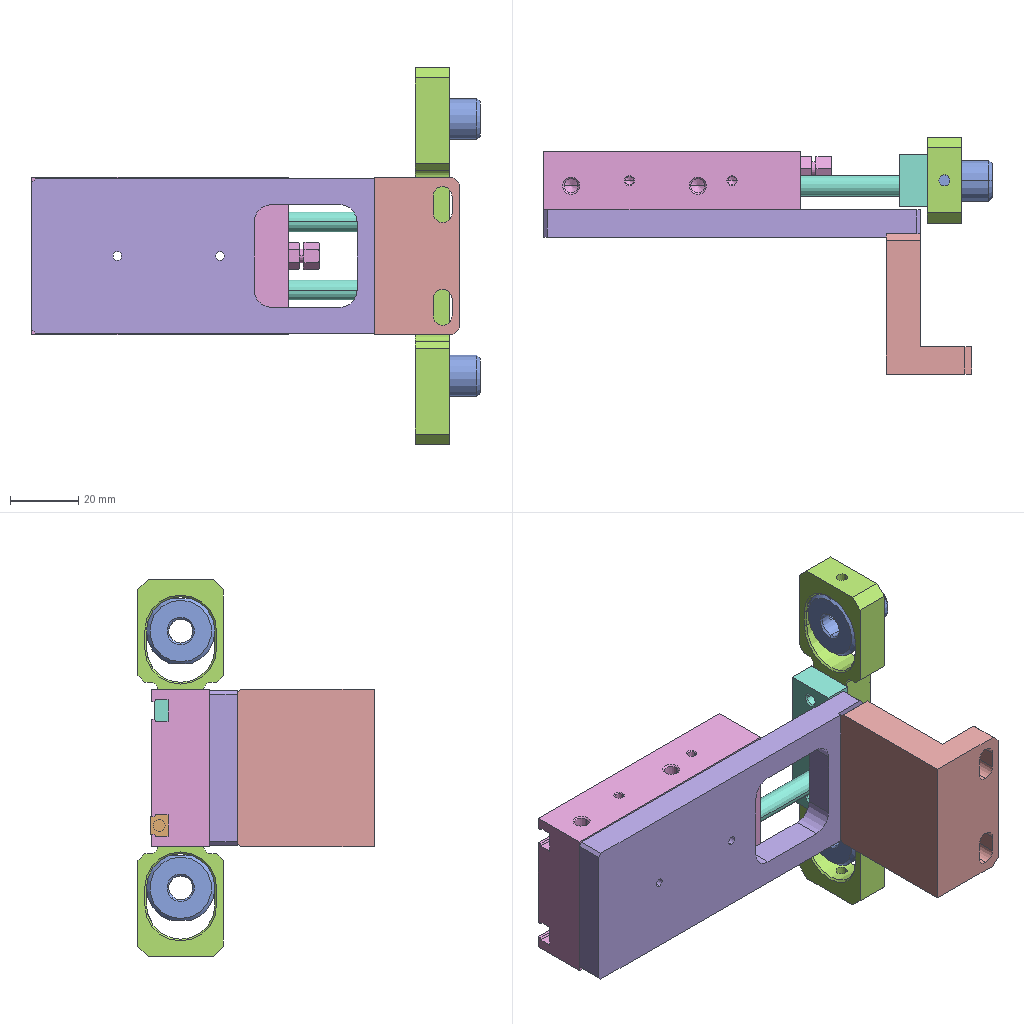Assembly | SolidWorks | 9 different items | 10 placed | box 131 x 69 x 110 mm
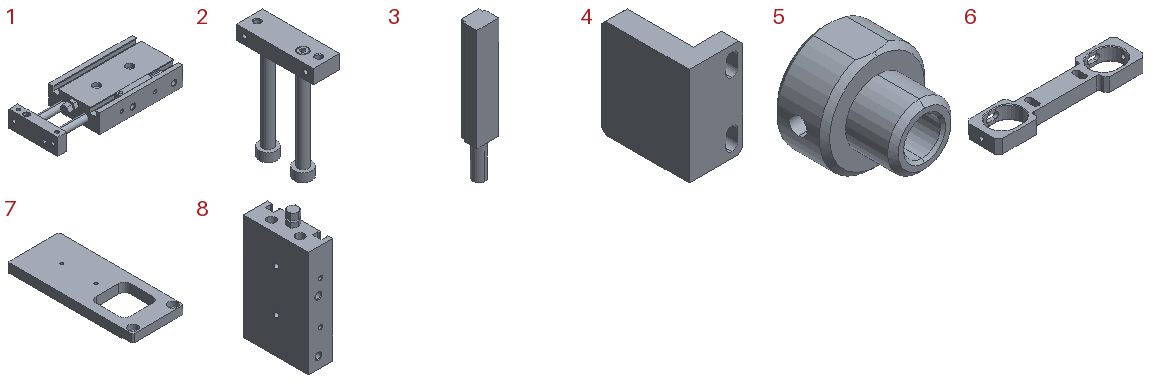Parts list (item | name | quantity | parent item | size | volume | features):
1 | (subassembly) | x1 | - | 112 x 46 x 17.2 mm | 58274 mm3 | features AEMSimFeature 1
2 | - | x1 | in 1 | 15 x 44 x 62 mm | 8556 mm3 | features HoleWzd 4, ICE 4, RefAxis 3, RevCut 2, Revolution 2, 3DProfileFeature 1, Extrusion 1
3 | - | x1 | in 1 | 6.2 x 5 x 39 mm | 946.118 mm3 | features RefAxis 6, 3DProfileFeature 2, Extrusion 1, RevCut 1, Revolution 1
4 | - | x1 | - | 25 x 41 x 46 mm | 23309 mm3 | features Chamfer 1, Extrusion 1, HoleWzd 1, ICE 1
5 | - | x2 | - | 20 x 19 x 19 mm | 3253 mm3 | features Chamfer 2, HoleWzd 2, ICE 1, Revolution 1
6 | - | x1 | - | 110 x 25 x 10 mm | 11689 mm3 | features ICE 5, Chamfer 3, HoleWzd 2, Extrusion 1, Fillet 1
7 | - | x1 | - | 45 x 110 x 8 mm | 31489 mm3 | features HoleWzd 2, ICE 2, Chamfer 1, Extrusion 1
8 | - | x1 | in 1 | 17 x 46 x 84 mm | 48772 mm3 | features HoleWzd 10, RefAxis 9, RevCut 4, 3DProfileFeature 3, Revolution 2, Extrusion 1, ICE 1
9 | YWC070U-12M-04 | x1 | - | - | - | -
Mates (type | each side: item.copy, entity, surface, feature):
In the top assembly
Coincident | 5.1 face plane Revolve1 | 6.1 face plane Boss-Extrude1
Coincident | 5.2 face plane Revolve1 | 6.1 face plane Boss-Extrude1
Parallel | 6.1 face plane Boss-Extrude1 | 5.2 plane
Parallel | 6.1 face plane Boss-Extrude1 | 5.1 plane
Tangent | 5.2 face cylinder Revolve1 | 6.1 face plane Cut-Extrude1
Tangent | 5.1 face cylinder Revolve1 | 6.1 face plane Cut-Extrude1
LimitDistanceDim | 6.1 face plane Boss-Extrude1 | 5.2 plane
LimitDistanceDim | 5.1 plane | 6.1 face plane Boss-Extrude1
Coincident | 6.1 face plane Boss-Extrude1 | 2.1 face plane Boss-Extrude1
Width | 6.1 face plane Boss-Extrude1 | 6.1 face plane Boss-Extrude1 | 2.1 face plane Boss-Extrude1 | 2.1 face plane Boss-Extrude1
Width | 6.1 face plane Cut-Extrude2 | 6.1 face plane Cut-Extrude2 | 2.1 face cylinder Cut-Revolve1
Coincident | 8.1 face plane Boss-Extrude1 | 7.1 face plane Boss-Extrude1
Concentric | 8.1 face cylinder Hole1 | 7.1 face cylinder M3 Tapped Hole1
Concentric | 8.1 face cylinder Hole2 | 7.1 face cylinder M3 Tapped Hole1
Concentric | 4.1 face cylinder M4 Tapped Hole1 | 7.1 face cylinder Hole size (% based on socket head cap screw type)1 | 2 times
Coincident | 4.1 face plane Boss-Extrude1 | 7.1 face plane Cut-Extrude1
In subassembly 1
Coincident | 8.2 axis | 2.2 axis
PlanarAngleDim | 2.2 plane | 8.2 plane
Coincident | 8.2 axis | 3.1 axis
LimitDistanceDim | 2.2 face plane Revolve1 | 8.2 face plane Cut-Revolve1